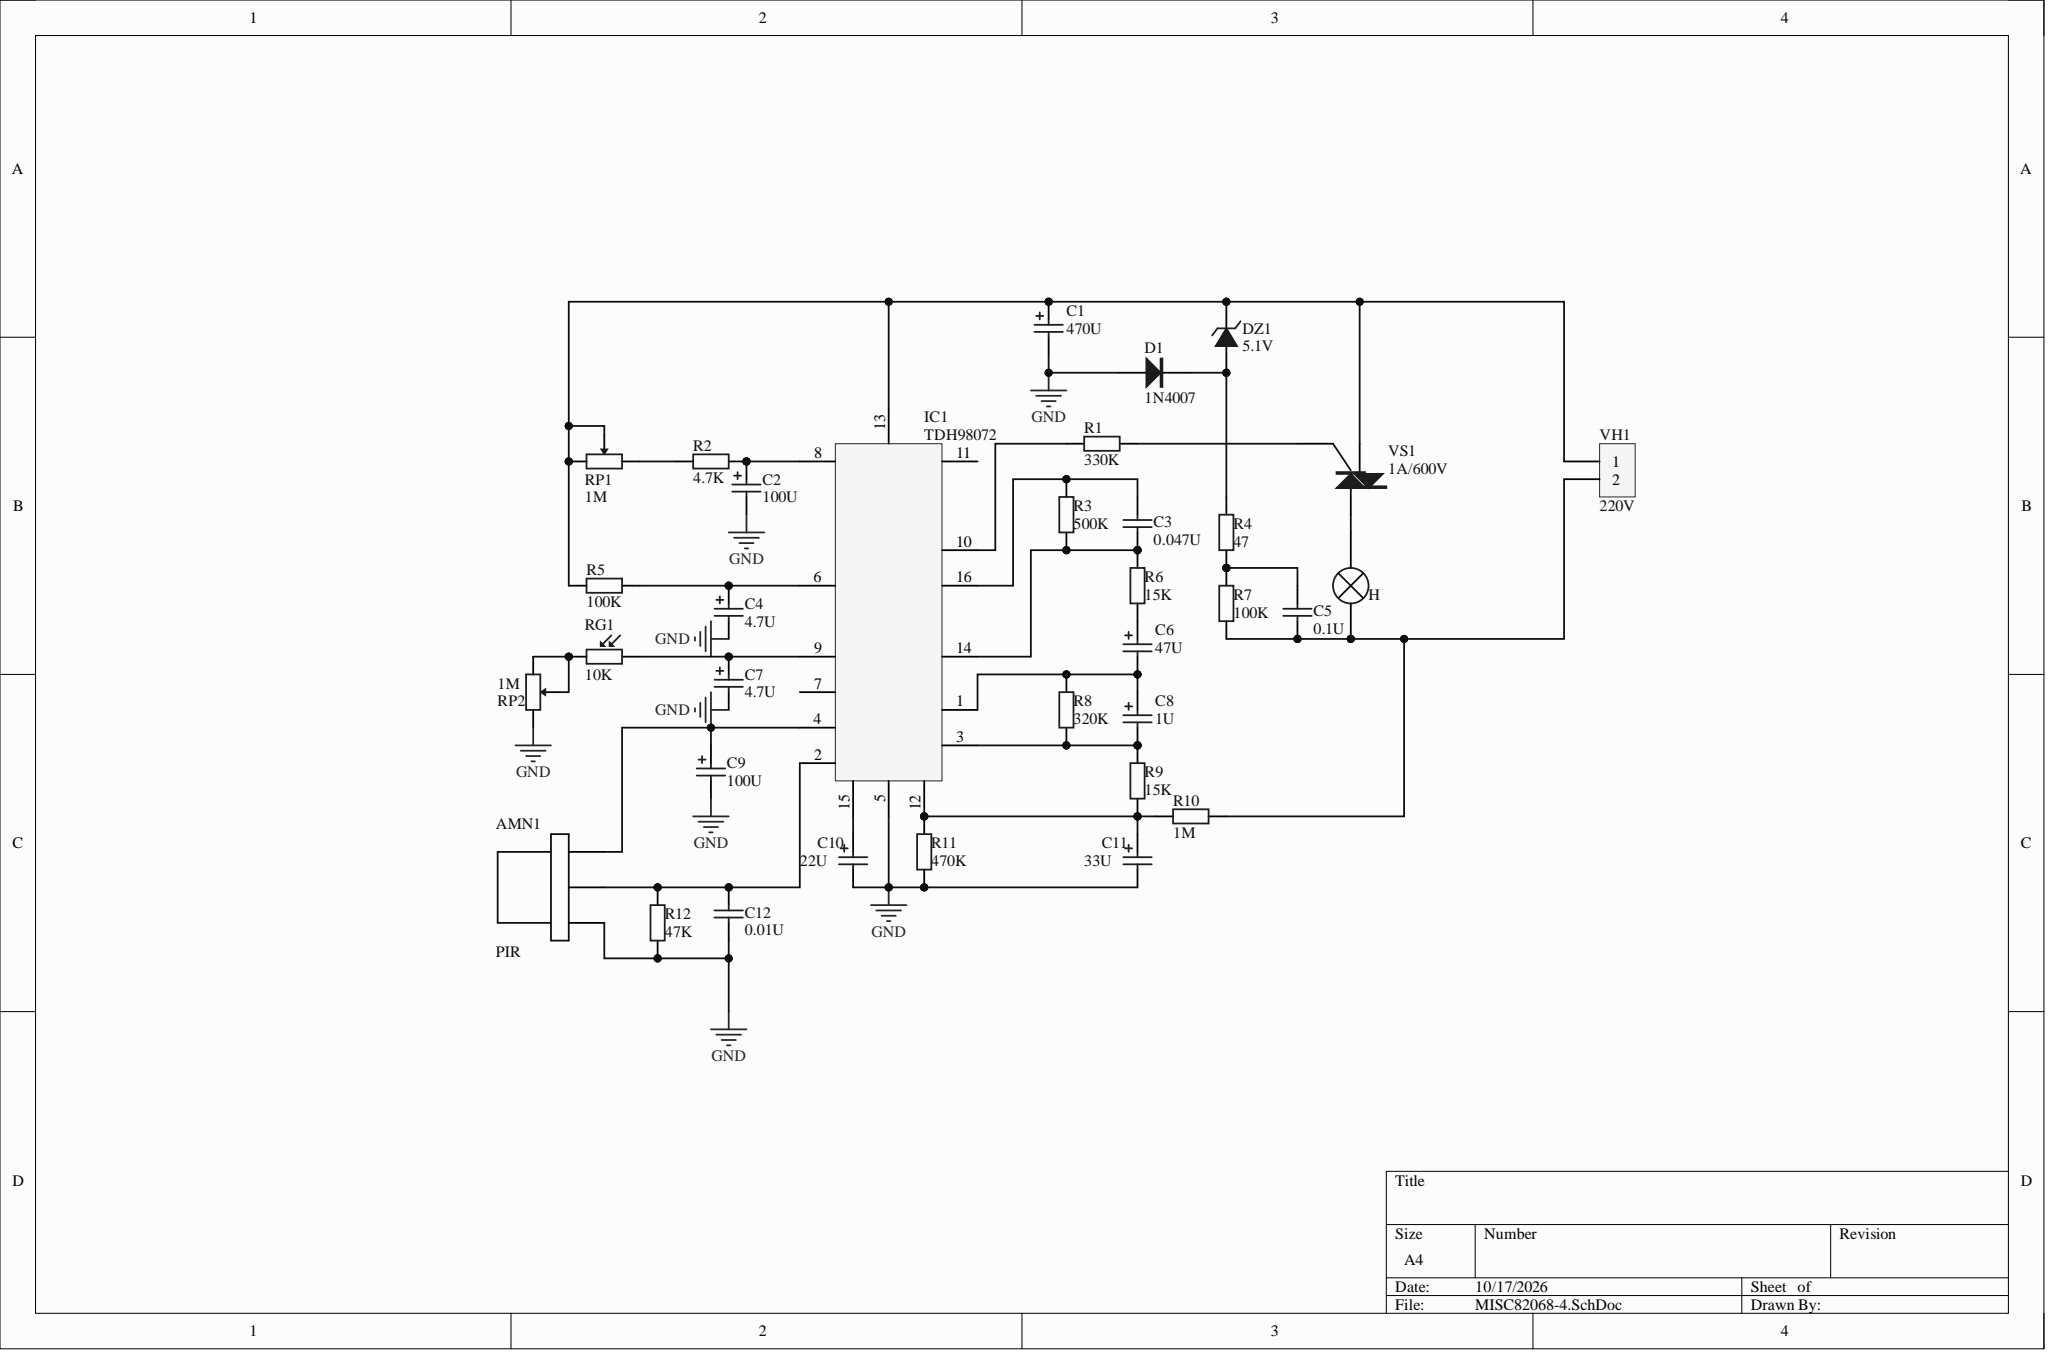Circuit board | Altium Designer | 34 parts | 22 nets
Bill of materials:
Comment,Description,Designator,Footprint,LibRef,Quantity
"H","","*1","HDR1X2","H","1"
"PIR","","AMN1","HDR1X3","PIR","1"
"470U","Polarized Capacitor (Axial)","C1","POLAR0.8","Cap Pol2","1"
"100U","Polarized Capacitor (Axial)","C2, C9","POLAR0.8","Cap Pol2","2"
"0.047U","Capacitor","C3","RAD-0.3","Cap","1"
"4.7U","Polarized Capacitor (Axial)","C4, C7","POLAR0.8","Cap Pol2","2"
"0.1U","Capacitor","C5","RAD-0.3","Cap","1"
"47U","Polarized Capacitor (Axial)","C6","POLAR0.8","Cap Pol2","1"
"1U","Polarized Capacitor (Axial)","C8","POLAR0.8","Cap Pol2","1"
"22U","Polarized Capacitor (Axial)","C10","POLAR0.8","Cap Pol2","1"
"33U","Polarized Capacitor (Axial)","C11","POLAR0.8","Cap Pol2","1"
"0.01U","Capacitor","C12","RAD-0.3","Cap","1"
"1N4007","Rectifier diode","D1","DO-41","1N4007","1"
"5.1V","3V/0.5W Zener diode","DZ1","DO-35","1N4619","1"
"TDH98072","","IC1","DIP16","TDH98072","1"
"330K","Resistor","R1","AXIAL-0.4","Res2","1"
"4.7K","Resistor","R2","AXIAL-0.4","Res2","1"
"500K","Resistor","R3","AXIAL-0.4","Res2","1"
"47","Resistor","R4","AXIAL-0.4","Res2","1"
"100K","Resistor","R5, R7","AXIAL-0.4","Res2","2"
"15K","Resistor","R6, R9","AXIAL-0.4","Res2","2"
"320K","Resistor","R8","AXIAL-0.4","Res2","1"
"1M","Resistor","R10","AXIAL-0.4","Res2","1"
"470K","Resistor","R11","AXIAL-0.4","Res2","1"
"47K","Resistor","R12","AXIAL-0.4","Res2","1"
"10K","Photoresistor","RG1","AXIAL-0.4","RG","1"
"1M","Single potentiometer","RP1, RP2","3296W","RP","2"
"220V","","VH1","VH3.96-2A","VH2","1"
"1A/600V","","VS1","LED 3mm-2P","1A/600V","1"
Netlist (Protel format):
[
*1
HDR1X2
H



]
[
AMN1
HDR1X3
PIR



]
[
C1
POLAR0.8
470U



]
[
C2
POLAR0.8
100U



]
[
C3
RAD-0.3
0.047U



]
[
C4
POLAR0.8
4.7U



]
[
C5
RAD-0.3
0.1U



]
[
C6
POLAR0.8
47U



]
[
C7
POLAR0.8
4.7U



]
[
C8
POLAR0.8
1U



]
[
C9
POLAR0.8
100U



]
[
C10
POLAR0.8
22U



]
[
C11
POLAR0.8
33U



]
[
C12
RAD-0.3
0.01U



]
[
D1
DO-41
1N4007



]
[
DZ1
DO-35
5.1V



]
[
IC1
DIP16
TDH98072



]
[
R1
AXIAL-0.4
330K



]
[
R2
AXIAL-0.4
4.7K



]
[
R3
AXIAL-0.4
500K



]
[
R4
AXIAL-0.4
47



]
[
R5
AXIAL-0.4
100K



]
[
R6
AXIAL-0.4
15K



]
[
R7
AXIAL-0.4
100K



]
[
R8
AXIAL-0.4
320K



]
[
R9
AXIAL-0.4
15K



]
[
R10
AXIAL-0.4
1M



]
[
R11
AXIAL-0.4
470K



]
[
R12
AXIAL-0.4
47K



]
[
RG1
AXIAL-0.4
10K



]
[
RP1
3296W
1M



]
[
RP2
3296W
1M



]
[
VH1
VH3.96-2A
220V



]
[
VS1
LED 3mm-2P
1A/600V



]
(
NetRG1_2
RG1-2
RP2-1
RP2-2
)
(
NetR2_1
R2-1
RP1-3
)
(
NetR1_1
R1-1
VS1-3
)
(
NetIC1_10
IC1-10
R1-2
)
(
NetD1_2
D1-2
DZ1-1
R4-2
)
(
NetC11_1
C11-1
IC1-12
R9-1
R10-1
R11-2
)
(
NetC10_1
C10-1
IC1-15
)
(
NetC8_2
C8-2
IC1-3
R8-1
R9-2
)
(
NetC7_1
C7-1
IC1-9
RG1-1
)
(
NetC6_2
C6-2
C8-1
IC1-1
R8-2
)
(
NetC6_1
C6-1
R6-1
)
(
NetC5_2
C5-2
R4-1
R7-2
)
(
NetC4_1
C4-1
IC1-6
R5-2
)
(
NetC3_2
C3-2
IC1-16
R3-2
)
(
NetC3_1
C3-1
IC1-14
R3-1
R6-2
)
(
NetC2_1
C2-1
IC1-8
R2-2
)
(
NetC1_1
C1-1
DZ1-2
IC1-13
R5-1
RP1-1
RP1-2
VH1-1
VS1-2
)
(
NetAMN1_2
AMN1-2
C12-2
IC1-2
R12-2
)
(
NetAMN1_1
AMN1-1
C9-1
IC1-4
)
(
Net*1_2
*1-2
C5-1
R7-1
R10-2
VH1-2
)
(
Net*1_1
*1-1
VS1-1
)
(
GND
AMN1-3
C1-2
C2-2
C4-2
C7-2
C9-2
C10-2
C11-2
C12-1
D1-1
IC1-5
R11-1
R12-1
RP2-3
)